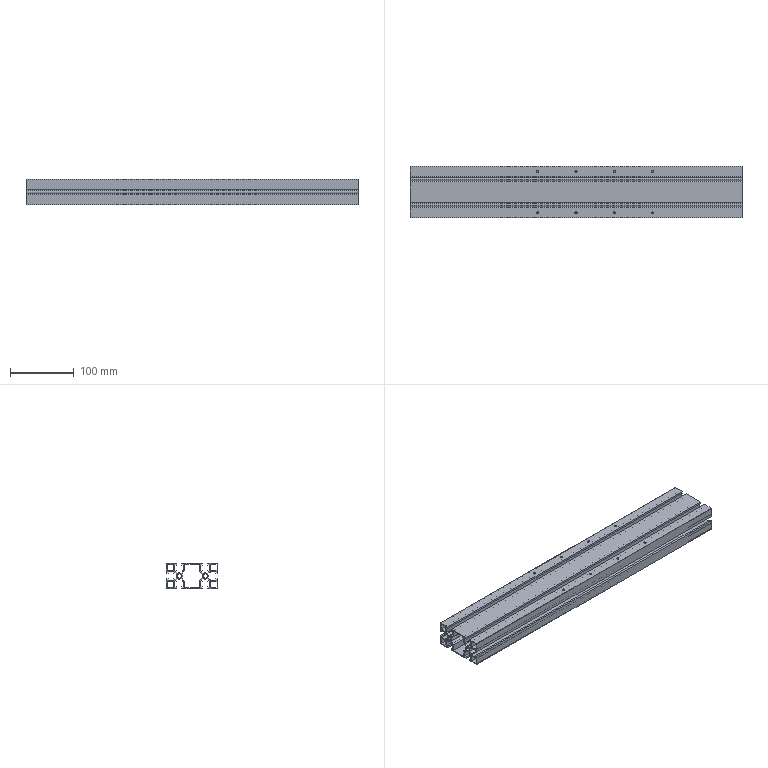Part | 1 solid | 142 faces | box 520 x 80 x 40 mm | volume 360577 mm3 | plane 110 | cylinder 32 | commonest cylinder face diameters 3.3 x16 9.6 x10 6.6 x4 0.6 x2